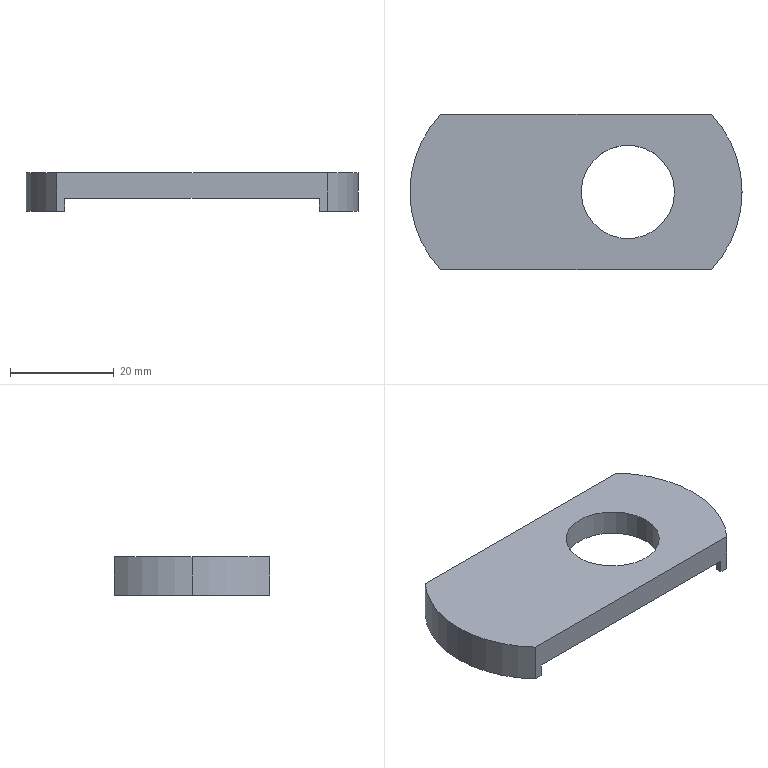Part | SolidWorks | features ICE 5, 3DProfileFeature 2, HoleWzd 2, Extrusion 1 | 1 solid | 37 faces | box 64 x 30 x 7.5 mm | volume 7628 mm3 | cylinder 18 | plane 11 | cone 8 | commonest cylinder face diameters 0.8 x8 40.2 x3 44 x3 17 x2 18 x2
STEP:
#1=CARTESIAN_POINT('',(-16.,14.,2.4));
#2=VERTEX_POINT('',#1);
#3=CARTESIAN_POINT('',(-16.,14.,3.2));
#4=VERTEX_POINT('',#3);
#5=CARTESIAN_POINT('',(-16.,14.,2.8));
#6=DIRECTION('',(0.,1.,0.));
#7=DIRECTION('',(0.,0.,1.));
#8=AXIS2_PLACEMENT_3D('',#5,#6,#7);
#9=CIRCLE('',#8,0.4);
#10=EDGE_CURVE('',#2,#4,#9,.T.);
#11=ORIENTED_EDGE('',*,*,#10,.F.);
#12=CARTESIAN_POINT('',(-16.,15.,2.4));
#13=VERTEX_POINT('',#12);
#14=CARTESIAN_POINT('',(-16.,15.,2.4));
#15=DIRECTION('',(0.,1.,0.));
#16=VECTOR('',#15,1000.);
#17=LINE('',#14,#16);
#18=EDGE_CURVE('',#2,#13,#17,.T.);
#19=ORIENTED_EDGE('',*,*,#18,.T.);
#20=CARTESIAN_POINT('',(-16.,15.,3.2));
#21=VERTEX_POINT('',#20);
#22=CARTESIAN_POINT('',(-16.,15.,2.8));
#23=DIRECTION('',(0.,1.,0.));
#24=DIRECTION('',(0.,0.,1.));
#25=AXIS2_PLACEMENT_3D('',#22,#23,#24);
#26=CIRCLE('',#25,0.4);
#27=EDGE_CURVE('',#13,#21,#26,.T.);
#28=ORIENTED_EDGE('',*,*,#27,.T.);
#29=CARTESIAN_POINT('',(-16.,15.,3.2));
#30=DIRECTION('',(0.,1.,0.));
#31=VECTOR('',#30,1000.);
#32=LINE('',#29,#31);
#33=EDGE_CURVE('',#4,#21,#32,.T.);
#34=ORIENTED_EDGE('',*,*,#33,.F.);
#35=EDGE_LOOP('',(#11,#19,#28,#34));
#36=FACE_OUTER_BOUND('',#35,.T.);
#37=CARTESIAN_POINT('',(-16.,15.,2.8));
#38=DIRECTION('',(0.,1.,0.));
#39=DIRECTION('',(0.,0.,1.));
#40=AXIS2_PLACEMENT_3D('',#37,#38,#39);
#41=CYLINDRICAL_SURFACE('',#40,0.4);
#42=ADVANCED_FACE('',(#36),#41,.F.);
#43=CARTESIAN_POINT('',(-16.,13.76,2.8));
#44=VERTEX_POINT('',#43);
#45=CARTESIAN_POINT('',(-16.,14.,3.2));
#46=DIRECTION('',(0.,0.515,0.8572));
#47=VECTOR('',#46,1000.);
#48=LINE('',#45,#47);
#49=EDGE_CURVE('',#44,#4,#48,.T.);
#50=ORIENTED_EDGE('',*,*,#49,.F.);
#51=CARTESIAN_POINT('',(-16.,14.,2.4));
#52=DIRECTION('',(0.,0.515,-0.8572));
#53=VECTOR('',#52,1000.);
#54=LINE('',#51,#53);
#55=EDGE_CURVE('',#44,#2,#54,.T.);
#56=ORIENTED_EDGE('',*,*,#55,.T.);
#57=ORIENTED_EDGE('',*,*,#10,.T.);
#58=EDGE_LOOP('',(#50,#56,#57));
#59=FACE_OUTER_BOUND('',#58,.T.);
#60=CARTESIAN_POINT('',(-16.,14.,2.8));
#61=DIRECTION('',(0.,1.,0.));
#62=DIRECTION('',(0.,0.,1.));
#63=AXIS2_PLACEMENT_3D('',#60,#61,#62);
#64=CONICAL_SURFACE('',#63,0.4,1.03);
#65=ADVANCED_FACE('',(#59),#64,.F.);
#66=CARTESIAN_POINT('',(4.,14.,2.4));
#67=VERTEX_POINT('',#66);
#68=CARTESIAN_POINT('',(4.,14.,3.2));
#69=VERTEX_POINT('',#68);
#70=CARTESIAN_POINT('',(4.,14.,2.8));
#71=DIRECTION('',(0.,1.,0.));
#72=DIRECTION('',(0.,0.,1.));
#73=AXIS2_PLACEMENT_3D('',#70,#71,#72);
#74=CIRCLE('',#73,0.4);
#75=EDGE_CURVE('',#67,#69,#74,.T.);
#76=ORIENTED_EDGE('',*,*,#75,.F.);
#77=CARTESIAN_POINT('',(4.,15.,2.4));
#78=VERTEX_POINT('',#77);
#79=CARTESIAN_POINT('',(4.,15.,2.4));
#80=DIRECTION('',(0.,1.,0.));
#81=VECTOR('',#80,1000.);
#82=LINE('',#79,#81);
#83=EDGE_CURVE('',#67,#78,#82,.T.);
#84=ORIENTED_EDGE('',*,*,#83,.T.);
#85=CARTESIAN_POINT('',(4.,15.,3.2));
#86=VERTEX_POINT('',#85);
#87=CARTESIAN_POINT('',(4.,15.,2.8));
#88=DIRECTION('',(0.,1.,0.));
#89=DIRECTION('',(0.,0.,1.));
#90=AXIS2_PLACEMENT_3D('',#87,#88,#89);
#91=CIRCLE('',#90,0.4);
#92=EDGE_CURVE('',#78,#86,#91,.T.);
#93=ORIENTED_EDGE('',*,*,#92,.T.);
#94=CARTESIAN_POINT('',(4.,15.,3.2));
#95=DIRECTION('',(0.,1.,0.));
#96=VECTOR('',#95,1000.);
#97=LINE('',#94,#96);
#98=EDGE_CURVE('',#69,#86,#97,.T.);
#99=ORIENTED_EDGE('',*,*,#98,.F.);
#100=EDGE_LOOP('',(#76,#84,#93,#99));
#101=FACE_OUTER_BOUND('',#100,.T.);
#102=CARTESIAN_POINT('',(4.,15.,2.8));
#103=DIRECTION('',(0.,1.,0.));
#104=DIRECTION('',(0.,0.,1.));
#105=AXIS2_PLACEMENT_3D('',#102,#103,#104);
#106=CYLINDRICAL_SURFACE('',#105,0.4);
#107=ADVANCED_FACE('',(#101),#106,.F.);
#108=CARTESIAN_POINT('',(4.,13.76,2.8));
#109=VERTEX_POINT('',#108);
#110=CARTESIAN_POINT('',(4.,14.,3.2));
#111=DIRECTION('',(0.,0.515,0.8572));
#112=VECTOR('',#111,1000.);
#113=LINE('',#110,#112);
#114=EDGE_CURVE('',#109,#69,#113,.T.);
#115=ORIENTED_EDGE('',*,*,#114,.F.);
#116=CARTESIAN_POINT('',(4.,14.,2.4));
#117=DIRECTION('',(0.,0.515,-0.8572));
#118=VECTOR('',#117,1000.);
#119=LINE('',#116,#118);
#120=EDGE_CURVE('',#109,#67,#119,.T.);
#121=ORIENTED_EDGE('',*,*,#120,.T.);
#122=ORIENTED_EDGE('',*,*,#75,.T.);
#123=EDGE_LOOP('',(#115,#121,#122));
#124=FACE_OUTER_BOUND('',#123,.T.);
#125=CARTESIAN_POINT('',(4.,14.,2.8));
#126=DIRECTION('',(0.,1.,0.));
#127=DIRECTION('',(0.,0.,1.));
#128=AXIS2_PLACEMENT_3D('',#125,#126,#127);
#129=CONICAL_SURFACE('',#128,0.4,1.03);
#130=ADVANCED_FACE('',(#124),#129,.F.);
#131=CARTESIAN_POINT('',(1.4,12.5,1.));
#132=VERTEX_POINT('',#131);
#133=CARTESIAN_POINT('',(0.6,12.5,1.));
#134=VERTEX_POINT('',#133);
#135=CARTESIAN_POINT('',(1.,12.5,1.));
#136=DIRECTION('',(0.,0.,-1.));
#137=DIRECTION('',(-1.,0.,0.));
#138=AXIS2_PLACEMENT_3D('',#135,#136,#137);
#139=CIRCLE('',#138,0.4);
#140=EDGE_CURVE('',#132,#134,#139,.T.);
#141=ORIENTED_EDGE('',*,*,#140,.F.);
#142=CARTESIAN_POINT('',(1.4,12.5,0.));
#143=VERTEX_POINT('',#142);
#144=CARTESIAN_POINT('',(1.4,12.5,0.));
#145=DIRECTION('',(0.,0.,-1.));
#146=VECTOR('',#145,1000.);
#147=LINE('',#144,#146);
#148=EDGE_CURVE('',#132,#143,#147,.T.);
#149=ORIENTED_EDGE('',*,*,#148,.T.);
#150=CARTESIAN_POINT('',(0.6,12.5,0.));
#151=VERTEX_POINT('',#150);
#152=CARTESIAN_POINT('',(1.,12.5,0.));
#153=DIRECTION('',(0.,0.,-1.));
#154=DIRECTION('',(-1.,0.,0.));
#155=AXIS2_PLACEMENT_3D('',#152,#153,#154);
#156=CIRCLE('',#155,0.4);
#157=EDGE_CURVE('',#143,#151,#156,.T.);
#158=ORIENTED_EDGE('',*,*,#157,.T.);
#159=CARTESIAN_POINT('',(0.6,12.5,0.));
#160=DIRECTION('',(0.,0.,-1.));
#161=VECTOR('',#160,1000.);
#162=LINE('',#159,#161);
#163=EDGE_CURVE('',#134,#151,#162,.T.);
#164=ORIENTED_EDGE('',*,*,#163,.F.);
#165=EDGE_LOOP('',(#141,#149,#158,#164));
#166=FACE_OUTER_BOUND('',#165,.T.);
#167=CARTESIAN_POINT('',(1.,12.5,0.));
#168=DIRECTION('',(0.,0.,-1.));
#169=DIRECTION('',(-1.,0.,0.));
#170=AXIS2_PLACEMENT_3D('',#167,#168,#169);
#171=CYLINDRICAL_SURFACE('',#170,0.4);
#172=ADVANCED_FACE('',(#166),#171,.F.);
#173=CARTESIAN_POINT('',(1.,12.5,1.24));
#174=VERTEX_POINT('',#173);
#175=CARTESIAN_POINT('',(0.6,12.5,1.));
#176=DIRECTION('',(-0.8572,0.,-0.515));
#177=VECTOR('',#176,1000.);
#178=LINE('',#175,#177);
#179=EDGE_CURVE('',#174,#134,#178,.T.);
#180=ORIENTED_EDGE('',*,*,#179,.F.);
#181=CARTESIAN_POINT('',(1.4,12.5,1.));
#182=DIRECTION('',(0.8572,0.,-0.515));
#183=VECTOR('',#182,1000.);
#184=LINE('',#181,#183);
#185=EDGE_CURVE('',#174,#132,#184,.T.);
#186=ORIENTED_EDGE('',*,*,#185,.T.);
#187=ORIENTED_EDGE('',*,*,#140,.T.);
#188=EDGE_LOOP('',(#180,#186,#187));
#189=FACE_OUTER_BOUND('',#188,.T.);
#190=CARTESIAN_POINT('',(1.,12.5,1.));
#191=DIRECTION('',(0.,0.,-1.));
#192=DIRECTION('',(-1.,0.,0.));
#193=AXIS2_PLACEMENT_3D('',#190,#191,#192);
#194=CONICAL_SURFACE('',#193,0.4,1.03);
#195=ADVANCED_FACE('',(#189),#194,.F.);
#196=CARTESIAN_POINT('',(21.4,12.5,1.));
#197=VERTEX_POINT('',#196);
#198=CARTESIAN_POINT('',(20.6,12.5,1.));
#199=VERTEX_POINT('',#198);
#200=CARTESIAN_POINT('',(21.,12.5,1.));
#201=DIRECTION('',(0.,0.,-1.));
#202=DIRECTION('',(-1.,0.,0.));
#203=AXIS2_PLACEMENT_3D('',#200,#201,#202);
#204=CIRCLE('',#203,0.4);
#205=EDGE_CURVE('',#197,#199,#204,.T.);
#206=ORIENTED_EDGE('',*,*,#205,.F.);
#207=CARTESIAN_POINT('',(21.4,12.5,0.));
#208=VERTEX_POINT('',#207);
#209=CARTESIAN_POINT('',(21.4,12.5,0.));
#210=DIRECTION('',(0.,0.,-1.));
#211=VECTOR('',#210,1000.);
#212=LINE('',#209,#211);
#213=EDGE_CURVE('',#197,#208,#212,.T.);
#214=ORIENTED_EDGE('',*,*,#213,.T.);
#215=CARTESIAN_POINT('',(20.6,12.5,0.));
#216=VERTEX_POINT('',#215);
#217=CARTESIAN_POINT('',(21.,12.5,0.));
#218=DIRECTION('',(0.,0.,-1.));
#219=DIRECTION('',(-1.,0.,0.));
#220=AXIS2_PLACEMENT_3D('',#217,#218,#219);
#221=CIRCLE('',#220,0.4);
#222=EDGE_CURVE('',#208,#216,#221,.T.);
#223=ORIENTED_EDGE('',*,*,#222,.T.);
#224=CARTESIAN_POINT('',(20.6,12.5,0.));
#225=DIRECTION('',(0.,0.,-1.));
#226=VECTOR('',#225,1000.);
#227=LINE('',#224,#226);
#228=EDGE_CURVE('',#199,#216,#227,.T.);
#229=ORIENTED_EDGE('',*,*,#228,.F.);
#230=EDGE_LOOP('',(#206,#214,#223,#229));
#231=FACE_OUTER_BOUND('',#230,.T.);
#232=CARTESIAN_POINT('',(21.,12.5,0.));
#233=DIRECTION('',(0.,0.,-1.));
#234=DIRECTION('',(-1.,0.,0.));
#235=AXIS2_PLACEMENT_3D('',#232,#233,#234);
#236=CYLINDRICAL_SURFACE('',#235,0.4);
#237=ADVANCED_FACE('',(#231),#236,.F.);
#238=CARTESIAN_POINT('',(21.,12.5,1.24));
#239=VERTEX_POINT('',#238);
#240=CARTESIAN_POINT('',(20.6,12.5,1.));
#241=DIRECTION('',(-0.8572,0.,-0.515));
#242=VECTOR('',#241,1000.);
#243=LINE('',#240,#242);
#244=EDGE_CURVE('',#239,#199,#243,.T.);
#245=ORIENTED_EDGE('',*,*,#244,.F.);
#246=CARTESIAN_POINT('',(21.4,12.5,1.));
#247=DIRECTION('',(0.8572,0.,-0.515));
#248=VECTOR('',#247,1000.);
#249=LINE('',#246,#248);
#250=EDGE_CURVE('',#239,#197,#249,.T.);
#251=ORIENTED_EDGE('',*,*,#250,.T.);
#252=ORIENTED_EDGE('',*,*,#205,.T.);
#253=EDGE_LOOP('',(#245,#251,#252));
#254=FACE_OUTER_BOUND('',#253,.T.);
#255=CARTESIAN_POINT('',(21.,12.5,1.));
#256=DIRECTION('',(0.,0.,-1.));
#257=DIRECTION('',(-1.,0.,0.));
#258=AXIS2_PLACEMENT_3D('',#255,#256,#257);
#259=CONICAL_SURFACE('',#258,0.4,1.03);
#260=ADVANCED_FACE('',(#254),#259,.F.);
#261=CARTESIAN_POINT('',(19.,0.,5.));
#262=VERTEX_POINT('',#261);
#263=CARTESIAN_POINT('',(1.,0.,5.));
#264=VERTEX_POINT('',#263);
#265=CARTESIAN_POINT('',(10.,0.,5.));
#266=DIRECTION('',(0.,0.,-1.));
#267=DIRECTION('',(1.,0.,0.));
#268=AXIS2_PLACEMENT_3D('',#265,#266,#267);
#269=CIRCLE('',#268,9.);
#270=EDGE_CURVE('',#262,#264,#269,.T.);
#271=ORIENTED_EDGE('',*,*,#270,.F.);
#272=CARTESIAN_POINT('',(19.,0.,0.));
#273=VERTEX_POINT('',#272);
#274=CARTESIAN_POINT('',(19.,0.,5.001));
#275=DIRECTION('',(0.,0.,-1.));
#276=VECTOR('',#275,1000.);
#277=LINE('',#274,#276);
#278=EDGE_CURVE('',#262,#273,#277,.T.);
#279=ORIENTED_EDGE('',*,*,#278,.T.);
#280=CARTESIAN_POINT('',(1.,0.,0.));
#281=VERTEX_POINT('',#280);
#282=CARTESIAN_POINT('',(10.,0.,0.));
#283=DIRECTION('',(0.,0.,-1.));
#284=DIRECTION('',(-1.,0.,0.));
#285=AXIS2_PLACEMENT_3D('',#282,#283,#284);
#286=CIRCLE('',#285,9.);
#287=EDGE_CURVE('',#273,#281,#286,.T.);
#288=ORIENTED_EDGE('',*,*,#287,.T.);
#289=CARTESIAN_POINT('',(1.,0.,5.001));
#290=DIRECTION('',(0.,0.,-1.));
#291=VECTOR('',#290,1000.);
#292=LINE('',#289,#291);
#293=EDGE_CURVE('',#264,#281,#292,.T.);
#294=ORIENTED_EDGE('',*,*,#293,.F.);
#295=EDGE_LOOP('',(#271,#279,#288,#294));
#296=FACE_OUTER_BOUND('',#295,.T.);
#297=CARTESIAN_POINT('',(10.,0.,5.001));
#298=DIRECTION('',(0.,0.,-1.));
#299=DIRECTION('',(-1.,0.,0.));
#300=AXIS2_PLACEMENT_3D('',#297,#298,#299);
#301=CYLINDRICAL_SURFACE('',#300,9.);
#302=ADVANCED_FACE('',(#296),#301,.F.);
#303=CARTESIAN_POINT('',(-1.5,0.,2.));
#304=VERTEX_POINT('',#303);
#305=CARTESIAN_POINT('',(-18.5,0.,2.));
#306=VERTEX_POINT('',#305);
#307=CARTESIAN_POINT('',(-10.,0.,2.));
#308=DIRECTION('',(0.,0.,-1.));
#309=DIRECTION('',(-1.,0.,0.));
#310=AXIS2_PLACEMENT_3D('',#307,#308,#309);
#311=CIRCLE('',#310,8.5);
#312=EDGE_CURVE('',#304,#306,#311,.T.);
#313=ORIENTED_EDGE('',*,*,#312,.F.);
#314=CARTESIAN_POINT('',(-1.5,0.,0.));
#315=VERTEX_POINT('',#314);
#316=CARTESIAN_POINT('',(-1.5,0.,2.));
#317=DIRECTION('',(0.,0.,-1.));
#318=VECTOR('',#317,1000.);
#319=LINE('',#316,#318);
#320=EDGE_CURVE('',#304,#315,#319,.T.);
#321=ORIENTED_EDGE('',*,*,#320,.T.);
#322=CARTESIAN_POINT('',(-18.5,0.,0.));
#323=VERTEX_POINT('',#322);
#324=CARTESIAN_POINT('',(-10.,0.,0.));
#325=DIRECTION('',(0.,0.,-1.));
#326=DIRECTION('',(-1.,0.,0.));
#327=AXIS2_PLACEMENT_3D('',#324,#325,#326);
#328=CIRCLE('',#327,8.5);
#329=EDGE_CURVE('',#315,#323,#328,.T.);
#330=ORIENTED_EDGE('',*,*,#329,.T.);
#331=CARTESIAN_POINT('',(-18.5,0.,2.));
#332=DIRECTION('',(0.,0.,-1.));
#333=VECTOR('',#332,1000.);
#334=LINE('',#331,#333);
#335=EDGE_CURVE('',#306,#323,#334,.T.);
#336=ORIENTED_EDGE('',*,*,#335,.F.);
#337=EDGE_LOOP('',(#313,#321,#330,#336));
#338=FACE_OUTER_BOUND('',#337,.T.);
#339=CARTESIAN_POINT('',(-10.,0.,2.));
#340=DIRECTION('',(0.,0.,-1.));
#341=DIRECTION('',(-1.,0.,0.));
#342=AXIS2_PLACEMENT_3D('',#339,#340,#341);
#343=CYLINDRICAL_SURFACE('',#342,8.5);
#344=ADVANCED_FACE('',(#338),#343,.F.);
#345=CARTESIAN_POINT('',(-32.,0.,5.));
#346=VERTEX_POINT('',#345);
#347=CARTESIAN_POINT('',(-26.093,-15.,5.));
#348=VERTEX_POINT('',#347);
#349=CARTESIAN_POINT('',(-10.,0.,5.));
#350=DIRECTION('',(0.,0.,1.));
#351=DIRECTION('',(1.,0.,0.));
#352=AXIS2_PLACEMENT_3D('',#349,#350,#351);
#353=CIRCLE('',#352,22.);
#354=EDGE_CURVE('',#346,#348,#353,.T.);
#355=ORIENTED_EDGE('',*,*,#354,.F.);
#356=CARTESIAN_POINT('',(-32.,0.,-2.5));
#357=VERTEX_POINT('',#356);
#358=CARTESIAN_POINT('',(-32.,0.,5.));
#359=DIRECTION('',(0.,0.,-1.));
#360=VECTOR('',#359,1000.);
#361=LINE('',#358,#360);
#362=EDGE_CURVE('',#346,#357,#361,.T.);
#363=ORIENTED_EDGE('',*,*,#362,.T.);
#364=CARTESIAN_POINT('',(-26.093,-15.,-2.5));
#365=VERTEX_POINT('',#364);
#366=CARTESIAN_POINT('',(-10.,0.,-2.5));
#367=DIRECTION('',(0.,0.,-1.));
#368=DIRECTION('',(-1.,0.,0.));
#369=AXIS2_PLACEMENT_3D('',#366,#367,#368);
#370=CIRCLE('',#369,22.);
#371=EDGE_CURVE('',#365,#357,#370,.T.);
#372=ORIENTED_EDGE('',*,*,#371,.F.);
#373=CARTESIAN_POINT('',(-26.093,-15.,5.));
#374=DIRECTION('',(0.,0.,-1.));
#375=VECTOR('',#374,1000.);
#376=LINE('',#373,#375);
#377=EDGE_CURVE('',#348,#365,#376,.T.);
#378=ORIENTED_EDGE('',*,*,#377,.F.);
#379=EDGE_LOOP('',(#355,#363,#372,#378));
#380=FACE_OUTER_BOUND('',#379,.T.);
#381=CARTESIAN_POINT('',(-10.,0.,5.));
#382=DIRECTION('',(0.,0.,-1.));
#383=DIRECTION('',(-1.,0.,0.));
#384=AXIS2_PLACEMENT_3D('',#381,#382,#383);
#385=CYLINDRICAL_SURFACE('',#384,22.);
#386=ADVANCED_FACE('',(#380),#385,.T.);
#387=CARTESIAN_POINT('',(24.5,13.92,-2.5));
#388=VERTEX_POINT('',#387);
#389=CARTESIAN_POINT('',(30.1,0.,-2.5));
#390=VERTEX_POINT('',#389);
#391=CARTESIAN_POINT('',(10.,0.,-2.5));
#392=DIRECTION('',(0.,0.,-1.));
#393=DIRECTION('',(-1.,0.,0.));
#394=AXIS2_PLACEMENT_3D('',#391,#392,#393);
#395=CIRCLE('',#394,20.1);
#396=EDGE_CURVE('',#388,#390,#395,.T.);
#397=ORIENTED_EDGE('',*,*,#396,.T.);
#398=CARTESIAN_POINT('',(30.1,0.,0.));
#399=VERTEX_POINT('',#398);
#400=CARTESIAN_POINT('',(30.1,0.,-2.5));
#401=DIRECTION('',(0.,0.,1.));
#402=VECTOR('',#401,1000.);
#403=LINE('',#400,#402);
#404=EDGE_CURVE('',#390,#399,#403,.T.);
#405=ORIENTED_EDGE('',*,*,#404,.T.);
#406=CARTESIAN_POINT('',(24.5,13.92,0.));
#407=VERTEX_POINT('',#406);
#408=CARTESIAN_POINT('',(10.,0.,0.));
#409=DIRECTION('',(0.,0.,-1.));
#410=DIRECTION('',(-1.,0.,0.));
#411=AXIS2_PLACEMENT_3D('',#408,#409,#410);
#412=CIRCLE('',#411,20.1);
#413=EDGE_CURVE('',#407,#399,#412,.T.);
#414=ORIENTED_EDGE('',*,*,#413,.F.);
#415=CARTESIAN_POINT('',(24.5,13.92,-2.5));
#416=DIRECTION('',(0.,0.,-1.));
#417=VECTOR('',#416,1000.);
#418=LINE('',#415,#417);
#419=EDGE_CURVE('',#407,#388,#418,.T.);
#420=ORIENTED_EDGE('',*,*,#419,.T.);
#421=EDGE_LOOP('',(#397,#405,#414,#420));
#422=FACE_OUTER_BOUND('',#421,.T.);
#423=CARTESIAN_POINT('',(10.,0.,-2.5));
#424=DIRECTION('',(0.,0.,1.));
#425=DIRECTION('',(1.,0.,0.));
#426=AXIS2_PLACEMENT_3D('',#423,#424,#425);
#427=CYLINDRICAL_SURFACE('',#426,20.1);
#428=ADVANCED_FACE('',(#422),#427,.F.);
#429=CARTESIAN_POINT('',(24.5,-15.,-2.5));
#430=VERTEX_POINT('',#429);
#431=CARTESIAN_POINT('',(24.5,-15.,0.));
#432=VERTEX_POINT('',#431);
#433=CARTESIAN_POINT('',(24.5,-15.,5.));
#434=DIRECTION('',(0.,0.,1.));
#435=VECTOR('',#434,1000.);
#436=LINE('',#433,#435);
#437=EDGE_CURVE('',#430,#432,#436,.T.);
#438=ORIENTED_EDGE('',*,*,#437,.F.);
#439=CARTESIAN_POINT('',(26.093,-15.,-2.5));
#440=VERTEX_POINT('',#439);
#441=CARTESIAN_POINT('',(0.,-15.,-2.5));
#442=DIRECTION('',(-1.,0.,0.));
#443=VECTOR('',#442,1000.);
#444=LINE('',#441,#443);
#445=EDGE_CURVE('',#440,#430,#444,.T.);
#446=ORIENTED_EDGE('',*,*,#445,.F.);
#447=CARTESIAN_POINT('',(26.093,-15.,5.));
#448=VERTEX_POINT('',#447);
#449=CARTESIAN_POINT('',(26.093,-15.,5.));
#450=DIRECTION('',(0.,0.,-1.));
#451=VECTOR('',#450,1000.);
#452=LINE('',#449,#451);
#453=EDGE_CURVE('',#448,#440,#452,.T.);
#454=ORIENTED_EDGE('',*,*,#453,.F.);
#455=CARTESIAN_POINT('',(-26.093,-15.,5.));
#456=DIRECTION('',(1.,0.,0.));
#457=VECTOR('',#456,1000.);
#458=LINE('',#455,#457);
#459=EDGE_CURVE('',#348,#448,#458,.T.);
#460=ORIENTED_EDGE('',*,*,#459,.F.);
#461=ORIENTED_EDGE('',*,*,#377,.T.);
#462=CARTESIAN_POINT('',(-24.5,-15.,-2.5));
#463=VERTEX_POINT('',#462);
#464=CARTESIAN_POINT('',(0.,-15.,-2.5));
#465=DIRECTION('',(-1.,0.,0.));
#466=VECTOR('',#465,1000.);
#467=LINE('',#464,#466);
#468=EDGE_CURVE('',#463,#365,#467,.T.);
#469=ORIENTED_EDGE('',*,*,#468,.F.);
#470=CARTESIAN_POINT('',(-24.5,-15.,0.));
#471=VERTEX_POINT('',#470);
#472=CARTESIAN_POINT('',(-24.5,-15.,5.));
#473=DIRECTION('',(0.,0.,-1.));
#474=VECTOR('',#473,1000.);
#475=LINE('',#472,#474);
#476=EDGE_CURVE('',#471,#463,#475,.T.);
#477=ORIENTED_EDGE('',*,*,#476,.F.);
#478=CARTESIAN_POINT('',(-26.093,-15.,0.));
#479=DIRECTION('',(1.,0.,0.));
#480=VECTOR('',#479,1000.);
#481=LINE('',#478,#480);
#482=EDGE_CURVE('',#471,#432,#481,.T.);
#483=ORIENTED_EDGE('',*,*,#482,.T.);
#484=EDGE_LOOP('',(#438,#446,#454,#460,#461,#469,#477,#483));
#485=FACE_OUTER_BOUND('',#484,.T.);
#486=CARTESIAN_POINT('',(-26.093,-15.,5.));
#487=DIRECTION('',(0.,1.,0.));
#488=DIRECTION('',(-1.,0.,0.));
#489=AXIS2_PLACEMENT_3D('',#486,#487,#488);
#490=PLANE('',#489);
#491=ADVANCED_FACE('',(#485),#490,.F.);
#492=CARTESIAN_POINT('',(-16.,15.,2.8));
#493=DIRECTION('',(0.,1.,0.));
#494=DIRECTION('',(0.,0.,1.));
#495=AXIS2_PLACEMENT_3D('',#492,#493,#494);
#496=CIRCLE('',#495,0.4);
#497=EDGE_CURVE('',#21,#13,#496,.T.);
#498=ORIENTED_EDGE('',*,*,#497,.F.);
#499=ORIENTED_EDGE('',*,*,#27,.F.);
#500=EDGE_LOOP('',(#498,#499));
#501=FACE_BOUND('',#500,.T.);
#502=CARTESIAN_POINT('',(4.,15.,2.8));
#503=DIRECTION('',(0.,1.,0.));
#504=DIRECTION('',(0.,0.,1.));
#505=AXIS2_PLACEMENT_3D('',#502,#503,#504);
#506=CIRCLE('',#505,0.4);
#507=EDGE_CURVE('',#86,#78,#506,.T.);
#508=ORIENTED_EDGE('',*,*,#507,.F.);
#509=ORIENTED_EDGE('',*,*,#92,.F.);
#510=EDGE_LOOP('',(#508,#509));
#511=FACE_BOUND('',#510,.T.);
#512=CARTESIAN_POINT('',(-24.5,15.,-2.5));
#513=VERTEX_POINT('',#512);
#514=CARTESIAN_POINT('',(-24.5,15.,0.));
#515=VERTEX_POINT('',#514);
#516=CARTESIAN_POINT('',(-24.5,15.,5.));
#517=DIRECTION('',(0.,0.,1.));
#518=VECTOR('',#517,1000.);
#519=LINE('',#516,#518);
#520=EDGE_CURVE('',#513,#515,#519,.T.);
#521=ORIENTED_EDGE('',*,*,#520,.F.);
#522=CARTESIAN_POINT('',(-26.093,15.,-2.5));
#523=VERTEX_POINT('',#522);
#524=CARTESIAN_POINT('',(0.,15.,-2.5));
#525=DIRECTION('',(1.,0.,0.));
#526=VECTOR('',#525,1000.);
#527=LINE('',#524,#526);
#528=EDGE_CURVE('',#523,#513,#527,.T.);
#529=ORIENTED_EDGE('',*,*,#528,.F.);
#530=CARTESIAN_POINT('',(-26.093,15.,5.));
#531=VERTEX_POINT('',#530);
#532=CARTESIAN_POINT('',(-26.093,15.,5.));
#533=DIRECTION('',(0.,0.,-1.));
#534=VECTOR('',#533,1000.);
#535=LINE('',#532,#534);
#536=EDGE_CURVE('',#531,#523,#535,.T.);
#537=ORIENTED_EDGE('',*,*,#536,.F.);
#538=CARTESIAN_POINT('',(26.093,15.,5.));
#539=VERTEX_POINT('',#538);
#540=CARTESIAN_POINT('',(-26.093,15.,5.));
#541=DIRECTION('',(-1.,0.,0.));
#542=VECTOR('',#541,1000.);
#543=LINE('',#540,#542);
#544=EDGE_CURVE('',#539,#531,#543,.T.);
#545=ORIENTED_EDGE('',*,*,#544,.F.);
#546=CARTESIAN_POINT('',(26.093,15.,-2.5));
#547=VERTEX_POINT('',#546);
#548=CARTESIAN_POINT('',(26.093,15.,5.));
#549=DIRECTION('',(0.,0.,-1.));
#550=VECTOR('',#549,1000.);
#551=LINE('',#548,#550);
#552=EDGE_CURVE('',#539,#547,#551,.T.);
#553=ORIENTED_EDGE('',*,*,#552,.T.);
#554=CARTESIAN_POINT('',(24.5,15.,-2.5));
#555=VERTEX_POINT('',#554);
#556=CARTESIAN_POINT('',(0.,15.,-2.5));
#557=DIRECTION('',(1.,0.,0.));
#558=VECTOR('',#557,1000.);
#559=LINE('',#556,#558);
#560=EDGE_CURVE('',#555,#547,#559,.T.);
#561=ORIENTED_EDGE('',*,*,#560,.F.);
#562=CARTESIAN_POINT('',(24.5,15.,0.));
#563=VERTEX_POINT('',#562);
#564=CARTESIAN_POINT('',(24.5,15.,5.));
#565=DIRECTION('',(0.,0.,-1.));
#566=VECTOR('',#565,1000.);
#567=LINE('',#564,#566);
#568=EDGE_CURVE('',#563,#555,#567,.T.);
#569=ORIENTED_EDGE('',*,*,#568,.F.);
#570=CARTESIAN_POINT('',(-26.093,15.,0.));
#571=DIRECTION('',(-1.,0.,0.));
#572=VECTOR('',#571,1000.);
#573=LINE('',#570,#572);
#574=EDGE_CURVE('',#563,#515,#573,.T.);
#575=ORIENTED_EDGE('',*,*,#574,.T.);
#576=EDGE_LOOP('',(#521,#529,#537,#545,#553,#561,#569,#575));
#577=FACE_OUTER_BOUND('',#576,.T.);
#578=CARTESIAN_POINT('',(-26.093,15.,5.));
#579=DIRECTION('',(0.,-1.,0.));
#580=DIRECTION('',(1.,0.,0.));
#581=AXIS2_PLACEMENT_3D('',#578,#579,#580);
#582=PLANE('',#581);
#583=ADVANCED_FACE('',(#501,#511,#577),#582,.F.);
#584=ORIENTED_EDGE('',*,*,#404,.F.);
#585=CARTESIAN_POINT('',(24.5,-13.92,-2.5));
#586=VERTEX_POINT('',#585);
#587=CARTESIAN_POINT('',(10.,0.,-2.5));
#588=DIRECTION('',(0.,0.,-1.));
#589=DIRECTION('',(-1.,0.,0.));
#590=AXIS2_PLACEMENT_3D('',#587,#588,#589);
#591=CIRCLE('',#590,20.1);
#592=EDGE_CURVE('',#390,#586,#591,.T.);
#593=ORIENTED_EDGE('',*,*,#592,.T.);
#594=CARTESIAN_POINT('',(24.5,-13.92,0.));
#595=VERTEX_POINT('',#594);
#596=CARTESIAN_POINT('',(24.5,-13.92,-2.5));
#597=DIRECTION('',(0.,0.,1.));
#598=VECTOR('',#597,1000.);
#599=LINE('',#596,#598);
#600=EDGE_CURVE('',#586,#595,#599,.T.);
#601=ORIENTED_EDGE('',*,*,#600,.T.);
#602=CARTESIAN_POINT('',(10.,0.,0.));
#603=DIRECTION('',(0.,0.,-1.));
#604=DIRECTION('',(-1.,0.,0.));
#605=AXIS2_PLACEMENT_3D('',#602,#603,#604);
#606=CIRCLE('',#605,20.1);
#607=EDGE_CURVE('',#399,#595,#606,.T.);
#608=ORIENTED_EDGE('',*,*,#607,.F.);
#609=EDGE_LOOP('',(#584,#593,#601,#608));
#610=FACE_OUTER_BOUND('',#609,.T.);
#611=CARTESIAN_POINT('',(10.,0.,-2.5));
#612=DIRECTION('',(0.,0.,1.));
#613=DIRECTION('',(1.,0.,0.));
#614=AXIS2_PLACEMENT_3D('',#611,#612,#613);
#615=CYLINDRICAL_SURFACE('',#614,20.1);
#616=ADVANCED_FACE('',(#610),#615,.F.);
#617=ORIENTED_EDGE('',*,*,#445,.T.);
#618=CARTESIAN_POINT('',(24.5,0.,-2.5));
#619=DIRECTION('',(0.,1.,0.));
#620=VECTOR('',#619,1000.);
#621=LINE('',#618,#620);
#622=EDGE_CURVE('',#430,#586,#621,.T.);
#623=ORIENTED_EDGE('',*,*,#622,.T.);
#624=ORIENTED_EDGE('',*,*,#592,.F.);
#625=ORIENTED_EDGE('',*,*,#396,.F.);
#626=CARTESIAN_POINT('',(24.5,0.,-2.5));
#627=DIRECTION('',(0.,1.,0.));
#628=VECTOR('',#627,1000.);
#629=LINE('',#626,#628);
#630=EDGE_CURVE('',#388,#555,#629,.T.);
#631=ORIENTED_EDGE('',*,*,#630,.T.);
#632=ORIENTED_EDGE('',*,*,#560,.T.);
#633=CARTESIAN_POINT('',(10.,0.,-2.5));
#634=DIRECTION('',(0.,0.,-1.));
#635=DIRECTION('',(-1.,0.,0.));
#636=AXIS2_PLACEMENT_3D('',#633,#634,#635);
#637=CIRCLE('',#636,22.);
#638=EDGE_CURVE('',#547,#440,#637,.T.);
#639=ORIENTED_EDGE('',*,*,#638,.T.);
#640=EDGE_LOOP('',(#617,#623,#624,#625,#631,#632,#639));
#641=FACE_OUTER_BOUND('',#640,.T.);
#642=CARTESIAN_POINT('',(0.,0.,-2.5));
#643=DIRECTION('',(0.,0.,-1.));
#644=DIRECTION('',(-1.,0.,0.));
#645=AXIS2_PLACEMENT_3D('',#642,#643,#644);
#646=PLANE('',#645);
#647=ADVANCED_FACE('',(#641),#646,.T.);
#648=CARTESIAN_POINT('',(-24.5,13.92,0.));
#649=VERTEX_POINT('',#648);
#650=CARTESIAN_POINT('',(-24.5,13.92,-2.5));
#651=VERTEX_POINT('',#650);
#652=CARTESIAN_POINT('',(-24.5,13.92,-2.5));
#653=DIRECTION('',(0.,0.,-1.));
#654=VECTOR('',#653,1000.);
#655=LINE('',#652,#654);
#656=EDGE_CURVE('',#649,#651,#655,.T.);
#657=ORIENTED_EDGE('',*,*,#656,.F.);
#658=CARTESIAN_POINT('',(-24.5,-13.92,0.));
#659=VERTEX_POINT('',#658);
#660=CARTESIAN_POINT('',(-10.,0.,0.));
#661=DIRECTION('',(0.,0.,1.));
#662=DIRECTION('',(-1.,0.,0.));
#663=AXIS2_PLACEMENT_3D('',#660,#661,#662);
#664=CIRCLE('',#663,20.1);
#665=EDGE_CURVE('',#649,#659,#664,.T.);
#666=ORIENTED_EDGE('',*,*,#665,.T.);
#667=CARTESIAN_POINT('',(-24.5,-13.92,-2.5));
#668=VERTEX_POINT('',#667);
#669=CARTESIAN_POINT('',(-24.5,-13.92,-2.5));
#670=DIRECTION('',(0.,0.,1.));
#671=VECTOR('',#670,1000.);
#672=LINE('',#669,#671);
#673=EDGE_CURVE('',#668,#659,#672,.T.);
#674=ORIENTED_EDGE('',*,*,#673,.F.);
#675=CARTESIAN_POINT('',(-10.,0.,-2.5));
#676=DIRECTION('',(0.,0.,1.));
#677=DIRECTION('',(-1.,0.,0.));
#678=AXIS2_PLACEMENT_3D('',#675,#676,#677);
#679=CIRCLE('',#678,20.1);
#680=EDGE_CURVE('',#651,#668,#679,.T.);
#681=ORIENTED_EDGE('',*,*,#680,.F.);
#682=EDGE_LOOP('',(#657,#666,#674,#681));
#683=FACE_OUTER_BOUND('',#682,.T.);
#684=CARTESIAN_POINT('',(-10.,0.,-2.5));
#685=DIRECTION('',(0.,0.,1.));
#686=DIRECTION('',(1.,0.,0.));
#687=AXIS2_PLACEMENT_3D('',#684,#685,#686);
#688=CYLINDRICAL_SURFACE('',#687,20.1);
#689=ADVANCED_FACE('',(#683),#688,.F.);
#690=ORIENTED_EDGE('',*,*,#528,.T.);
#691=CARTESIAN_POINT('',(-24.5,0.,-2.5));
#692=DIRECTION('',(0.,-1.,0.));
#693=VECTOR('',#692,1000.);
#694=LINE('',#691,#693);
#695=EDGE_CURVE('',#513,#651,#694,.T.);
#696=ORIENTED_EDGE('',*,*,#695,.T.);
#697=ORIENTED_EDGE('',*,*,#680,.T.);
#698=CARTESIAN_POINT('',(-24.5,0.,-2.5));
#699=DIRECTION('',(0.,-1.,0.));
#700=VECTOR('',#699,1000.);
#701=LINE('',#698,#700);
#702=EDGE_CURVE('',#668,#463,#701,.T.);
#703=ORIENTED_EDGE('',*,*,#702,.T.);
#704=ORIENTED_EDGE('',*,*,#468,.T.);
#705=ORIENTED_EDGE('',*,*,#371,.T.);
#706=CARTESIAN_POINT('',(-10.,0.,-2.5));
#707=DIRECTION('',(0.,0.,-1.));
#708=DIRECTION('',(-1.,0.,0.));
#709=AXIS2_PLACEMENT_3D('',#706,#707,#708);
#710=CIRCLE('',#709,22.);
#711=EDGE_CURVE('',#357,#523,#710,.T.);
#712=ORIENTED_EDGE('',*,*,#711,.T.);
#713=EDGE_LOOP('',(#690,#696,#697,#703,#704,#705,#712));
#714=FACE_OUTER_BOUND('',#713,.T.);
#715=CARTESIAN_POINT('',(0.,0.,-2.5));
#716=DIRECTION('',(0.,0.,-1.));
#717=DIRECTION('',(-1.,0.,0.));
#718=AXIS2_PLACEMENT_3D('',#715,#716,#717);
#719=PLANE('',#718);
#720=ADVANCED_FACE('',(#714),#719,.T.);
#721=CARTESIAN_POINT('',(1.,12.5,0.));
#722=DIRECTION('',(0.,0.,-1.));
#723=DIRECTION('',(-1.,0.,0.));
#724=AXIS2_PLACEMENT_3D('',#721,#722,#723);
#725=CIRCLE('',#724,0.4);
#726=EDGE_CURVE('',#151,#143,#725,.T.);
#727=ORIENTED_EDGE('',*,*,#726,.F.);
#728=ORIENTED_EDGE('',*,*,#157,.F.);
#729=EDGE_LOOP('',(#727,#728));
#730=FACE_BOUND('',#729,.T.);
#731=CARTESIAN_POINT('',(21.,12.5,0.));
#732=DIRECTION('',(0.,0.,-1.));
#733=DIRECTION('',(-1.,0.,0.));
#734=AXIS2_PLACEMENT_3D('',#731,#732,#733);
#735=CIRCLE('',#734,0.4);
#736=EDGE_CURVE('',#216,#208,#735,.T.);
#737=ORIENTED_EDGE('',*,*,#736,.F.);
#738=ORIENTED_EDGE('',*,*,#222,.F.);
#739=EDGE_LOOP('',(#737,#738));
#740=FACE_BOUND('',#739,.T.);
#741=CARTESIAN_POINT('',(-10.,0.,0.));
#742=DIRECTION('',(0.,0.,-1.));
#743=DIRECTION('',(-1.,0.,0.));
#744=AXIS2_PLACEMENT_3D('',#741,#742,#743);
#745=CIRCLE('',#744,8.5);
#746=EDGE_CURVE('',#323,#315,#745,.T.);
#747=ORIENTED_EDGE('',*,*,#746,.F.);
#748=ORIENTED_EDGE('',*,*,#329,.F.);
#749=EDGE_LOOP('',(#747,#748));
#750=FACE_BOUND('',#749,.T.);
#751=CARTESIAN_POINT('',(10.,0.,0.));
#752=DIRECTION('',(0.,0.,-1.));
#753=DIRECTION('',(-1.,0.,0.));
#754=AXIS2_PLACEMENT_3D('',#751,#752,#753);
#755=CIRCLE('',#754,9.);
#756=EDGE_CURVE('',#281,#273,#755,.T.);
#757=ORIENTED_EDGE('',*,*,#756,.F.);
#758=ORIENTED_EDGE('',*,*,#287,.F.);
#759=EDGE_LOOP('',(#757,#758));
#760=FACE_BOUND('',#759,.T.);
#761=ORIENTED_EDGE('',*,*,#482,.F.);
#762=CARTESIAN_POINT('',(-24.5,18.222,0.));
#763=DIRECTION('',(0.,1.,0.));
#764=VECTOR('',#763,1000.);
#765=LINE('',#762,#764);
#766=EDGE_CURVE('',#471,#659,#765,.T.);
#767=ORIENTED_EDGE('',*,*,#766,.T.);
#768=ORIENTED_EDGE('',*,*,#665,.F.);
#769=CARTESIAN_POINT('',(-24.5,18.222,0.));
#770=DIRECTION('',(0.,1.,0.));
#771=VECTOR('',#770,1000.);
#772=LINE('',#769,#771);
#773=EDGE_CURVE('',#649,#515,#772,.T.);
#774=ORIENTED_EDGE('',*,*,#773,.T.);
#775=ORIENTED_EDGE('',*,*,#574,.F.);
#776=CARTESIAN_POINT('',(24.5,18.222,0.));
#777=DIRECTION('',(0.,-1.,0.));
#778=VECTOR('',#777,1000.);
#779=LINE('',#776,#778);
#780=EDGE_CURVE('',#563,#407,#779,.T.);
#781=ORIENTED_EDGE('',*,*,#780,.T.);
#782=ORIENTED_EDGE('',*,*,#413,.T.);
#783=ORIENTED_EDGE('',*,*,#607,.T.);
#784=CARTESIAN_POINT('',(24.5,18.222,0.));
#785=DIRECTION('',(0.,-1.,0.));
#786=VECTOR('',#785,1000.);
#787=LINE('',#784,#786);
#788=EDGE_CURVE('',#595,#432,#787,.T.);
#789=ORIENTED_EDGE('',*,*,#788,.T.);
#790=EDGE_LOOP('',(#761,#767,#768,#774,#775,#781,#782,#783,#789));
#791=FACE_OUTER_BOUND('',#790,.T.);
#792=CARTESIAN_POINT('',(-10.,0.,0.));
#793=DIRECTION('',(0.,0.,1.));
#794=DIRECTION('',(1.,0.,0.));
#795=AXIS2_PLACEMENT_3D('',#792,#793,#794);
#796=PLANE('',#795);
#797=ADVANCED_FACE('',(#730,#740,#750,#760,#791),#796,.F.);
#798=CARTESIAN_POINT('',(10.,0.,5.));
#799=DIRECTION('',(0.,0.,-1.));
#800=DIRECTION('',(1.,0.,0.));
#801=AXIS2_PLACEMENT_3D('',#798,#799,#800);
#802=CIRCLE('',#801,9.);
#803=EDGE_CURVE('',#264,#262,#802,.T.);
#804=ORIENTED_EDGE('',*,*,#803,.T.);
#805=ORIENTED_EDGE('',*,*,#270,.T.);
#806=EDGE_LOOP('',(#804,#805));
#807=FACE_BOUND('',#806,.T.);
#808=CARTESIAN_POINT('',(-10.,0.,5.));
#809=DIRECTION('',(0.,0.,1.));
#810=DIRECTION('',(1.,0.,0.));
#811=AXIS2_PLACEMENT_3D('',#808,#809,#810);
#812=CIRCLE('',#811,22.);
#813=EDGE_CURVE('',#531,#346,#812,.T.);
#814=ORIENTED_EDGE('',*,*,#813,.T.);
#815=ORIENTED_EDGE('',*,*,#354,.T.);
#816=ORIENTED_EDGE('',*,*,#459,.T.);
#817=CARTESIAN_POINT('',(10.,0.,5.));
#818=DIRECTION('',(0.,0.,1.));
#819=DIRECTION('',(1.,0.,0.));
#820=AXIS2_PLACEMENT_3D('',#817,#818,#819);
#821=CIRCLE('',#820,22.);
#822=EDGE_CURVE('',#448,#539,#821,.T.);
#823=ORIENTED_EDGE('',*,*,#822,.T.);
#824=ORIENTED_EDGE('',*,*,#544,.T.);
#825=EDGE_LOOP('',(#814,#815,#816,#823,#824));
#826=FACE_OUTER_BOUND('',#825,.T.);
#827=CARTESIAN_POINT('',(-10.,0.,5.));
#828=DIRECTION('',(0.,0.,1.));
#829=DIRECTION('',(1.,0.,0.));
#830=AXIS2_PLACEMENT_3D('',#827,#828,#829);
#831=PLANE('',#830);
#832=ADVANCED_FACE('',(#807,#826),#831,.T.);
#833=ORIENTED_EDGE('',*,*,#362,.F.);
#834=ORIENTED_EDGE('',*,*,#813,.F.);
#835=ORIENTED_EDGE('',*,*,#536,.T.);
#836=ORIENTED_EDGE('',*,*,#711,.F.);
#837=EDGE_LOOP('',(#833,#834,#835,#836));
#838=FACE_OUTER_BOUND('',#837,.T.);
#839=CARTESIAN_POINT('',(-10.,0.,5.));
#840=DIRECTION('',(0.,0.,-1.));
#841=DIRECTION('',(-1.,0.,0.));
#842=AXIS2_PLACEMENT_3D('',#839,#840,#841);
#843=CYLINDRICAL_SURFACE('',#842,22.);
#844=ADVANCED_FACE('',(#838),#843,.T.);
#845=ORIENTED_EDGE('',*,*,#453,.T.);
#846=ORIENTED_EDGE('',*,*,#638,.F.);
#847=ORIENTED_EDGE('',*,*,#552,.F.);
#848=ORIENTED_EDGE('',*,*,#822,.F.);
#849=EDGE_LOOP('',(#845,#846,#847,#848));
#850=FACE_OUTER_BOUND('',#849,.T.);
#851=CARTESIAN_POINT('',(10.,0.,5.));
#852=DIRECTION('',(0.,0.,-1.));
#853=DIRECTION('',(-1.,0.,0.));
#854=AXIS2_PLACEMENT_3D('',#851,#852,#853);
#855=CYLINDRICAL_SURFACE('',#854,22.);
#856=ADVANCED_FACE('',(#850),#855,.T.);
#857=ORIENTED_EDGE('',*,*,#320,.F.);
#858=CARTESIAN_POINT('',(-10.,0.,2.));
#859=DIRECTION('',(0.,0.,-1.));
#860=DIRECTION('',(-1.,0.,0.));
#861=AXIS2_PLACEMENT_3D('',#858,#859,#860);
#862=CIRCLE('',#861,8.5);
#863=EDGE_CURVE('',#306,#304,#862,.T.);
#864=ORIENTED_EDGE('',*,*,#863,.F.);
#865=ORIENTED_EDGE('',*,*,#335,.T.);
#866=ORIENTED_EDGE('',*,*,#746,.T.);
#867=EDGE_LOOP('',(#857,#864,#865,#866));
#868=FACE_OUTER_BOUND('',#867,.T.);
#869=CARTESIAN_POINT('',(-10.,0.,2.));
#870=DIRECTION('',(0.,0.,-1.));
#871=DIRECTION('',(-1.,0.,0.));
#872=AXIS2_PLACEMENT_3D('',#869,#870,#871);
#873=CYLINDRICAL_SURFACE('',#872,8.5);
#874=ADVANCED_FACE('',(#868),#873,.F.);
#875=ORIENTED_EDGE('',*,*,#863,.T.);
#876=ORIENTED_EDGE('',*,*,#312,.T.);
#877=EDGE_LOOP('',(#875,#876));
#878=FACE_OUTER_BOUND('',#877,.T.);
#879=CARTESIAN_POINT('',(-10.,0.,2.));
#880=DIRECTION('',(0.,0.,-1.));
#881=DIRECTION('',(-1.,0.,0.));
#882=AXIS2_PLACEMENT_3D('',#879,#880,#881);
#883=PLANE('',#882);
#884=ADVANCED_FACE('',(#878),#883,.T.);
#885=ORIENTED_EDGE('',*,*,#278,.F.);
#886=ORIENTED_EDGE('',*,*,#803,.F.);
#887=ORIENTED_EDGE('',*,*,#293,.T.);
#888=ORIENTED_EDGE('',*,*,#756,.T.);
#889=EDGE_LOOP('',(#885,#886,#887,#888));
#890=FACE_OUTER_BOUND('',#889,.T.);
#891=CARTESIAN_POINT('',(10.,0.,5.001));
#892=DIRECTION('',(0.,0.,-1.));
#893=DIRECTION('',(-1.,0.,0.));
#894=AXIS2_PLACEMENT_3D('',#891,#892,#893);
#895=CYLINDRICAL_SURFACE('',#894,9.);
#896=ADVANCED_FACE('',(#890),#895,.F.);
#897=ORIENTED_EDGE('',*,*,#476,.T.);
#898=ORIENTED_EDGE('',*,*,#702,.F.);
#899=ORIENTED_EDGE('',*,*,#673,.T.);
#900=ORIENTED_EDGE('',*,*,#766,.F.);
#901=EDGE_LOOP('',(#897,#898,#899,#900));
#902=FACE_OUTER_BOUND('',#901,.T.);
#903=CARTESIAN_POINT('',(-24.5,18.222,-11.5));
#904=DIRECTION('',(1.,0.,0.));
#905=DIRECTION('',(0.,0.,-1.));
#906=AXIS2_PLACEMENT_3D('',#903,#904,#905);
#907=PLANE('',#906);
#908=ADVANCED_FACE('',(#902),#907,.T.);
#909=ORIENTED_EDGE('',*,*,#520,.T.);
#910=ORIENTED_EDGE('',*,*,#773,.F.);
#911=ORIENTED_EDGE('',*,*,#656,.T.);
#912=ORIENTED_EDGE('',*,*,#695,.F.);
#913=EDGE_LOOP('',(#909,#910,#911,#912));
#914=FACE_OUTER_BOUND('',#913,.T.);
#915=CARTESIAN_POINT('',(-24.5,18.222,-11.5));
#916=DIRECTION('',(1.,0.,0.));
#917=DIRECTION('',(0.,0.,-1.));
#918=AXIS2_PLACEMENT_3D('',#915,#916,#917);
#919=PLANE('',#918);
#920=ADVANCED_FACE('',(#914),#919,.T.);
#921=ORIENTED_EDGE('',*,*,#568,.T.);
#922=ORIENTED_EDGE('',*,*,#630,.F.);
#923=ORIENTED_EDGE('',*,*,#419,.F.);
#924=ORIENTED_EDGE('',*,*,#780,.F.);
#925=EDGE_LOOP('',(#921,#922,#923,#924));
#926=FACE_OUTER_BOUND('',#925,.T.);
#927=CARTESIAN_POINT('',(24.5,18.222,-11.5));
#928=DIRECTION('',(-1.,0.,0.));
#929=DIRECTION('',(0.,0.,1.));
#930=AXIS2_PLACEMENT_3D('',#927,#928,#929);
#931=PLANE('',#930);
#932=ADVANCED_FACE('',(#926),#931,.T.);
#933=ORIENTED_EDGE('',*,*,#437,.T.);
#934=ORIENTED_EDGE('',*,*,#788,.F.);
#935=ORIENTED_EDGE('',*,*,#600,.F.);
#936=ORIENTED_EDGE('',*,*,#622,.F.);
#937=EDGE_LOOP('',(#933,#934,#935,#936));
#938=FACE_OUTER_BOUND('',#937,.T.);
#939=CARTESIAN_POINT('',(24.5,18.222,-11.5));
#940=DIRECTION('',(-1.,0.,0.));
#941=DIRECTION('',(0.,0.,1.));
#942=AXIS2_PLACEMENT_3D('',#939,#940,#941);
#943=PLANE('',#942);
#944=ADVANCED_FACE('',(#938),#943,.T.);
#945=ORIENTED_EDGE('',*,*,#250,.F.);
#946=ORIENTED_EDGE('',*,*,#244,.T.);
#947=CARTESIAN_POINT('',(21.,12.5,1.));
#948=DIRECTION('',(0.,0.,-1.));
#949=DIRECTION('',(-1.,0.,0.));
#950=AXIS2_PLACEMENT_3D('',#947,#948,#949);
#951=CIRCLE('',#950,0.4);
#952=EDGE_CURVE('',#199,#197,#951,.T.);
#953=ORIENTED_EDGE('',*,*,#952,.T.);
#954=EDGE_LOOP('',(#945,#946,#953));
#955=FACE_OUTER_BOUND('',#954,.T.);
#956=CARTESIAN_POINT('',(21.,12.5,1.));
#957=DIRECTION('',(0.,0.,-1.));
#958=DIRECTION('',(-1.,0.,0.));
#959=AXIS2_PLACEMENT_3D('',#956,#957,#958);
#960=CONICAL_SURFACE('',#959,0.4,1.03);
#961=ADVANCED_FACE('',(#955),#960,.F.);
#962=ORIENTED_EDGE('',*,*,#213,.F.);
#963=ORIENTED_EDGE('',*,*,#952,.F.);
#964=ORIENTED_EDGE('',*,*,#228,.T.);
#965=ORIENTED_EDGE('',*,*,#736,.T.);
#966=EDGE_LOOP('',(#962,#963,#964,#965));
#967=FACE_OUTER_BOUND('',#966,.T.);
#968=CARTESIAN_POINT('',(21.,12.5,0.));
#969=DIRECTION('',(0.,0.,-1.));
#970=DIRECTION('',(-1.,0.,0.));
#971=AXIS2_PLACEMENT_3D('',#968,#969,#970);
#972=CYLINDRICAL_SURFACE('',#971,0.4);
#973=ADVANCED_FACE('',(#967),#972,.F.);
#974=ORIENTED_EDGE('',*,*,#185,.F.);
#975=ORIENTED_EDGE('',*,*,#179,.T.);
#976=CARTESIAN_POINT('',(1.,12.5,1.));
#977=DIRECTION('',(0.,0.,-1.));
#978=DIRECTION('',(-1.,0.,0.));
#979=AXIS2_PLACEMENT_3D('',#976,#977,#978);
#980=CIRCLE('',#979,0.4);
#981=EDGE_CURVE('',#134,#132,#980,.T.);
#982=ORIENTED_EDGE('',*,*,#981,.T.);
#983=EDGE_LOOP('',(#974,#975,#982));
#984=FACE_OUTER_BOUND('',#983,.T.);
#985=CARTESIAN_POINT('',(1.,12.5,1.));
#986=DIRECTION('',(0.,0.,-1.));
#987=DIRECTION('',(-1.,0.,0.));
#988=AXIS2_PLACEMENT_3D('',#985,#986,#987);
#989=CONICAL_SURFACE('',#988,0.4,1.03);
#990=ADVANCED_FACE('',(#984),#989,.F.);
#991=ORIENTED_EDGE('',*,*,#148,.F.);
#992=ORIENTED_EDGE('',*,*,#981,.F.);
#993=ORIENTED_EDGE('',*,*,#163,.T.);
#994=ORIENTED_EDGE('',*,*,#726,.T.);
#995=EDGE_LOOP('',(#991,#992,#993,#994));
#996=FACE_OUTER_BOUND('',#995,.T.);
#997=CARTESIAN_POINT('',(1.,12.5,0.));
#998=DIRECTION('',(0.,0.,-1.));
#999=DIRECTION('',(-1.,0.,0.));
#1000=AXIS2_PLACEMENT_3D('',#997,#998,#999);
#1001=CYLINDRICAL_SURFACE('',#1000,0.4);
#1002=ADVANCED_FACE('',(#996),#1001,.F.);
#1003=ORIENTED_EDGE('',*,*,#120,.F.);
#1004=ORIENTED_EDGE('',*,*,#114,.T.);
#1005=CARTESIAN_POINT('',(4.,14.,2.8));
#1006=DIRECTION('',(0.,1.,0.));
#1007=DIRECTION('',(0.,0.,1.));
#1008=AXIS2_PLACEMENT_3D('',#1005,#1006,#1007);
#1009=CIRCLE('',#1008,0.4);
#1010=EDGE_CURVE('',#69,#67,#1009,.T.);
#1011=ORIENTED_EDGE('',*,*,#1010,.T.);
#1012=EDGE_LOOP('',(#1003,#1004,#1011));
#1013=FACE_OUTER_BOUND('',#1012,.T.);
#1014=CARTESIAN_POINT('',(4.,14.,2.8));
#1015=DIRECTION('',(0.,1.,0.));
#1016=DIRECTION('',(0.,0.,1.));
#1017=AXIS2_PLACEMENT_3D('',#1014,#1015,#1016);
#1018=CONICAL_SURFACE('',#1017,0.4,1.03);
#1019=ADVANCED_FACE('',(#1013),#1018,.F.);
#1020=ORIENTED_EDGE('',*,*,#83,.F.);
#1021=ORIENTED_EDGE('',*,*,#1010,.F.);
#1022=ORIENTED_EDGE('',*,*,#98,.T.);
#1023=ORIENTED_EDGE('',*,*,#507,.T.);
#1024=EDGE_LOOP('',(#1020,#1021,#1022,#1023));
#1025=FACE_OUTER_BOUND('',#1024,.T.);
#1026=CARTESIAN_POINT('',(4.,15.,2.8));
#1027=DIRECTION('',(0.,1.,0.));
#1028=DIRECTION('',(0.,0.,1.));
#1029=AXIS2_PLACEMENT_3D('',#1026,#1027,#1028);
#1030=CYLINDRICAL_SURFACE('',#1029,0.4);
#1031=ADVANCED_FACE('',(#1025),#1030,.F.);
#1032=ORIENTED_EDGE('',*,*,#55,.F.);
#1033=ORIENTED_EDGE('',*,*,#49,.T.);
#1034=CARTESIAN_POINT('',(-16.,14.,2.8));
#1035=DIRECTION('',(0.,1.,0.));
#1036=DIRECTION('',(0.,0.,1.));
#1037=AXIS2_PLACEMENT_3D('',#1034,#1035,#1036);
#1038=CIRCLE('',#1037,0.4);
#1039=EDGE_CURVE('',#4,#2,#1038,.T.);
#1040=ORIENTED_EDGE('',*,*,#1039,.T.);
#1041=EDGE_LOOP('',(#1032,#1033,#1040));
#1042=FACE_OUTER_BOUND('',#1041,.T.);
#1043=CARTESIAN_POINT('',(-16.,14.,2.8));
#1044=DIRECTION('',(0.,1.,0.));
#1045=DIRECTION('',(0.,0.,1.));
#1046=AXIS2_PLACEMENT_3D('',#1043,#1044,#1045);
#1047=CONICAL_SURFACE('',#1046,0.4,1.03);
#1048=ADVANCED_FACE('',(#1042),#1047,.F.);
#1049=ORIENTED_EDGE('',*,*,#18,.F.);
#1050=ORIENTED_EDGE('',*,*,#1039,.F.);
#1051=ORIENTED_EDGE('',*,*,#33,.T.);
#1052=ORIENTED_EDGE('',*,*,#497,.T.);
#1053=EDGE_LOOP('',(#1049,#1050,#1051,#1052));
#1054=FACE_OUTER_BOUND('',#1053,.T.);
#1055=CARTESIAN_POINT('',(-16.,15.,2.8));
#1056=DIRECTION('',(0.,1.,0.));
#1057=DIRECTION('',(0.,0.,1.));
#1058=AXIS2_PLACEMENT_3D('',#1055,#1056,#1057);
#1059=CYLINDRICAL_SURFACE('',#1058,0.4);
#1060=ADVANCED_FACE('',(#1054),#1059,.F.);
#1061=CLOSED_SHELL('',(#42,#65,#107,#130,#172,#195,#237,#260,#302,#344,#386,#428,#491,#583,#616,#647,#689,#720,#797,#832,#844,#856,#874,#884,#896,#908,#920,#932,#944,#961,#973,#990,#1002,#1019,#1031,#1048,#1060));
#1062=MANIFOLD_SOLID_BREP('',#1061);
#1063=CARTESIAN_POINT('',(0.,0.,0.));
#1064=DIRECTION('',(0.,0.,1.));
#1065=DIRECTION('',(1.,0.,0.));
#1066=AXIS2_PLACEMENT_3D('',#1063,#1064,#1065);
#1067=(LENGTH_UNIT()NAMED_UNIT(*)SI_UNIT(.MILLI.,.METRE.));
#1068=UNCERTAINTY_MEASURE_WITH_UNIT(LENGTH_MEASURE(0.00001),#1067,'','');
#1069=(NAMED_UNIT(*)PLANE_ANGLE_UNIT()SI_UNIT($,.RADIAN.));
#1070=(NAMED_UNIT(*)SI_UNIT($,.STERADIAN.)SOLID_ANGLE_UNIT());
#1071=(GEOMETRIC_REPRESENTATION_CONTEXT(3)GLOBAL_UNCERTAINTY_ASSIGNED_CONTEXT((#1068))GLOBAL_UNIT_ASSIGNED_CONTEXT((#1067,#1069,#1070))REPRESENTATION_CONTEXT('',''));
#1072=ADVANCED_BREP_SHAPE_REPRESENTATION('',(#1062,#1066),#1071);